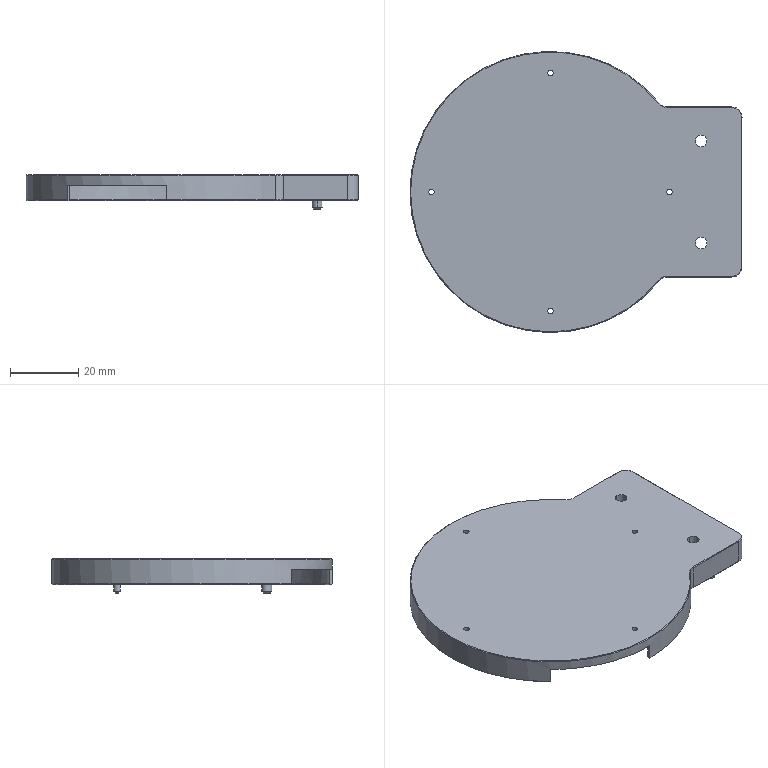NC program | NX | posted with a generic post | part box 97.6 x 82.6 x 10 mm
Lines 4683 to 4898 of 4898:
(PLANAR_MILL_COPY_COPY_COPY_COPY_COPY_COPY_1_COPY_1_1 , TOOL : D6A45)
N9346 T01 M6
N9348 G54
N9350 G17 G0 G90 X-27.416 Y-35.189 S9500 M3
N9352 G43 Z30. H1
N9354 Z-2.
N9356 G94 G1 Z-3.5 F1250.
N9358 X-26.755 Y-35.175
N9360 G3 X-25.9 Y-34.657 R1.
N9362 G1 Y-26.829
N9364 G3 X-26.673 Y-25.202 R2.1
N9366 G2 X29.767 Y37.412 R-42.2
N9368 X29.769 Y35.996 R1.
N9370 G1 X29.201 Y35.428
N9372 G2 X27.814 Y35.402 R1.
N9374 G3 X-38.465 Y16.028 R39.397
N9376 X13.475 Y-29.523 R39.399
N9378 X39.396 Y7.438 R39.391
N9380 G2 X40.395 Y8.4 R1.
N9382 G1 X41.2
N9384 G2 X42.2 Y7.398 R1.
N9386 X26.673 Y-25.202 R42.2
N9388 G3 X25.9 Y-26.829 R2.1
N9390 G1 Y-33.752
N9392 G3 X26.827 Y-34.126 R1.
N9394 G1 X27.492 Y-34.032
N9396 Z-2.
N9398 G0 Z30.
N9400 Y-39.568
N9402 Z-2.
N9404 G1 Z-3.5
N9406 X26.827 Y-39.474
N9408 G3 X25.9 Y-39.848 R1.
N9410 G1 Y-45.8
N9412 G2 X22. Y-49.7 R3.9
N9414 G1 X-22.
N9416 G2 X-25.9 Y-45.8 R3.9
N9418 G1 Y-38.943
N9420 G3 X-26.755 Y-38.425 R1.
N9422 G1 X-27.416 Y-38.411
N9424 Z-2.
N9426 G0 Z30.
N9428 X21.723 Y-30.656
N9430 Z-2.
N9432 G1 Z-3.5
N9434 X21.967 Y-31.282
N9436 G3 X22.748 Y-31.907 R1.
N9438 X23.1 Y-31.1 R1.1
N9440 G1 Y-29.795
N9442 G3 X21.441 Y-28.847 R1.1
N9444 G2 X17.164 Y-31.052 R42.2
N9446 G3 X17.408 Y-32.2 R0.6
N9448 G1 X20.172
N9450 G3 X20.792 Y-31.415 R1.
N9452 G1 X20.889 Y-30.751
N9454 Z-2.
N9456 G0 Z30.
N9458 X14.588 Y-37.489
N9460 Z-2.
N9462 G1 X14.779 Y-37.6 Z-2.059
N9464 X15.221 Z-2.178
N9466 X15.587 Y-37.387 Z-2.291
N9468 X15.8 Y-37.021 Z-2.405
N9470 Y-36.579 Z-2.523
N9472 X15.587 Y-36.213 Z-2.637
N9474 X15.221 Y-36. Z-2.75
N9476 X14.779 Z-2.869
N9478 X14.413 Y-36.213 Z-2.982
N9480 X14.2 Y-36.579 Z-3.095
N9482 Y-37.021 Z-3.214
N9484 X14.413 Y-37.387 Z-3.327
N9486 X14.779 Y-37.6 Z-3.441
N9488 X15. Z-3.5
N9490 G3 X15.8 Y-36.8 R0.8
N9492 X15. Y-37.6 R-0.8
N9494 X15.433 Y-37.35 R0.5
N9496 G1 Z-2.
N9498 G0 Z30.
N9500 X19.232 Y-42.292
N9502 Z-2.
N9504 G1 Z-3.5
N9506 X19.326 Y-41.627
N9508 G3 X18.952 Y-40.7 R1.
N9510 G1 X14.
N9512 G3 X11.9 Y-42.8 R2.1
N9514 G1 Y-44.8
N9516 G3 X14. Y-46.9 R2.1
N9518 G1 X21.5
N9520 G3 X23.1 Y-45.3 R1.6
N9522 G1 Y-42.8
N9524 G3 X22.781 Y-41.688 R2.1
N9526 X22.005 Y-42.318 R1.
N9528 G1 X21.765 Y-42.946
N9530 Z-2.
N9532 G0 Z30.
N9534 X-1.27 Y-45.7
N9536 Z-2.
N9538 G1 Z-3.5
N9540 X-0.866 Y-46.4
N9542 G3 X0. Y-46.9 R1.
N9544 G1 X7.
N9546 G3 X9.1 Y-44.8 R2.1
N9548 G1 Y-36.243
N9550 G3 X6.668 Y-34.17 R2.1
N9552 G2 X-6.668 Y-34.17 R42.2
N9554 G3 X-9.1 Y-36.243 R2.1
N9556 G1 Y-44.8
N9558 G3 X-7. Y-46.9 R2.1
N9560 G1 X0.
N9562 G3 X0.866 Y-46.4 R1.
N9564 G1 X1.27 Y-45.7
N9566 Z-2.
N9568 G0 Z30.
N9570 X-21.301 Y-42.407
N9572 Z-2.
N9574 G1 Z-3.5
N9576 X-21.579 Y-41.808
N9578 G3 X-22.397 Y-41.232 R1.
N9580 X-23.1 Y-42.8 R2.1
N9582 G1 Y-45.3
N9584 G3 X-21.5 Y-46.9 R1.6
N9586 G1 X-14.
N9588 G3 X-11.9 Y-44.8 R2.1
N9590 G1 Y-42.8
N9592 G3 X-14. Y-40.7 R2.1
N9594 G1 X-19.857
N9596 G3 X-20.375 Y-41.555 R1.
N9598 G1 X-20.389 Y-42.216
N9600 Z-2.
N9602 G0 Z30.
N9604 X-15.412 Y-37.489
N9606 Z-2.
N9608 G1 X-15.221 Y-37.6 Z-2.059
N9610 X-14.779 Z-2.178
N9612 X-14.413 Y-37.387 Z-2.291
N9614 X-14.2 Y-37.021 Z-2.405
N9616 Y-36.579 Z-2.523
N9618 X-14.413 Y-36.213 Z-2.637
N9620 X-14.779 Y-36. Z-2.75
N9622 X-15.221 Z-2.869
N9624 X-15.587 Y-36.213 Z-2.982
N9626 X-15.8 Y-36.579 Z-3.095
N9628 Y-37.021 Z-3.214
N9630 X-15.587 Y-37.387 Z-3.327
N9632 X-15.221 Y-37.6 Z-3.441
N9634 X-15. Z-3.5
N9636 G3 X-14.2 Y-36.8 R0.8
N9638 X-15. Y-37.6 R-0.8
N9640 X-14.567 Y-37.35 R0.5
N9642 G1 Z-2.
N9644 G0 Z30.
N9646 X-20.974 Y-31.
N9648 Z-2.
N9650 G1 Z-3.5
N9652 X-20.57 Y-31.7
N9654 G3 X-19.704 Y-32.2 R1.
N9656 G1 X-17.408
N9658 G3 X-17.164 Y-31.052 R0.6
N9660 G2 X-21.441 Y-28.847 R42.2
N9662 G3 X-23.1 Y-29.795 R1.1
N9664 G1 Y-31.1
N9666 G3 X-22. Y-32.2 R1.1
N9668 G1 X-19.704
N9670 G3 X-18.838 Y-31.7 R1.
N9672 G1 X-20.033 Y-31.
N9674 Z-2.
N9676 G0 Z30.
(DRILLING_COPY_1_COPY , TOOL : D6A45)
N9678 X0. Y42.5 S5000
N9680 G81 G98 Z-8.3 F350. R-4.
N9682 X-35. Y7.5
N9684 X0. Y-27.5
N9686 X35. Y7.5
N9688 G80
N9690 G0 X35. Y7.5 Z30.
(PLANAR_MILL_COPY_COPY_COPY_COPY_COPY_COPY_1_COPY_1_1_COPY , TOOL : D6A45)
N9692 X18.802 Y-37.954 S9500
N9694 Z0.5
N9696 G1 Z-1. F1250.
N9698 X19.3 Y-37.666
N9700 G3 X19.8 Y-36.8 R1.
N9702 G2 X22. Y-34.6 R2.2
N9704 X19.8 Y-36.8 R-2.2
N9706 G3 X19.3 Y-35.934 R1.
N9708 G1 X19.55 Y-37.666
N9710 G3 X20.05 Y-36.8 R1.
N9712 G2 X22. Y-34.85 R1.95
N9714 X20.05 Y-36.8 R-1.95
N9716 G3 X19.55 Y-35.934 R1.
N9718 G1 X18.847 Y-35.528
N9720 Z0.5
N9722 G0 Z30.
N9724 X-24.668 Y-37.936
N9726 Z0.5
N9728 G1 Z-1.
N9730 X-24.2 Y-37.666
N9732 G3 X-23.7 Y-36.8 R1.
N9734 G2 X-22. Y-35.1 R1.7
N9736 X-23.7 Y-36.8 R-1.7
N9738 G3 X-24.2 Y-35.934 R1.
N9740 G1 X-23.95 Y-37.666
N9742 G3 X-23.45 Y-36.8 R1.
N9744 G2 X-22. Y-35.35 R1.45
N9746 X-23.45 Y-36.8 R-1.45
N9748 G3 X-23.95 Y-35.934 R1.
N9750 G1 X-24.616 Y-35.549
N9752 Z0.5
N9754 G0 Z30.
N9756 M5
N9758 M2